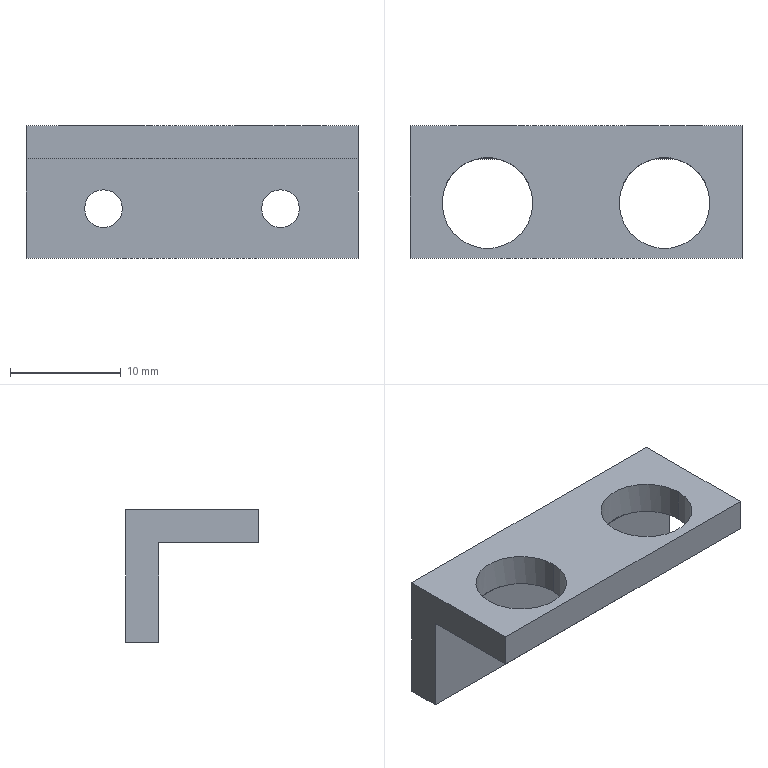Part | NX | 1 solid | 22 faces | box 30 x 12 x 12 mm | volume 1480 mm3 | plane 10 | cylinder 8 | cone 4 | commonest cylinder face diameters 3.4 x4 8.2 x4
STEP:
#1=CARTESIAN_POINT('',(-8.,4.34,-9.2));
#2=VERTEX_POINT('',#1);
#3=CARTESIAN_POINT('',(-8.,4.34,-5.8));
#4=VERTEX_POINT('',#3);
#5=CARTESIAN_POINT('',(-8.,4.34,-7.5));
#6=DIRECTION('',(0.,1.,0.));
#7=DIRECTION('',(0.,0.,1.));
#8=AXIS2_PLACEMENT_3D('',#5,#6,#7);
#9=CIRCLE('',#8,1.7);
#10=EDGE_CURVE('',#2,#4,#9,.T.);
#11=ORIENTED_EDGE('',*,*,#10,.F.);
#12=CARTESIAN_POINT('',(-8.,6.,-10.86));
#13=VERTEX_POINT('',#12);
#14=CARTESIAN_POINT('',(-8.,6.,-10.86));
#15=DIRECTION('',(0.,0.7071,-0.7071));
#16=VECTOR('',#15,1000.);
#17=LINE('',#14,#16);
#18=EDGE_CURVE('',#2,#13,#17,.T.);
#19=ORIENTED_EDGE('',*,*,#18,.T.);
#20=CARTESIAN_POINT('',(-8.,6.,-4.14));
#21=VERTEX_POINT('',#20);
#22=CARTESIAN_POINT('',(-8.,6.,-7.5));
#23=DIRECTION('',(0.,1.,0.));
#24=DIRECTION('',(0.,0.,1.));
#25=AXIS2_PLACEMENT_3D('',#22,#23,#24);
#26=CIRCLE('',#25,3.36);
#27=EDGE_CURVE('',#13,#21,#26,.T.);
#28=ORIENTED_EDGE('',*,*,#27,.T.);
#29=CARTESIAN_POINT('',(-8.,6.,-4.14));
#30=DIRECTION('',(0.,0.7071,0.7071));
#31=VECTOR('',#30,1000.);
#32=LINE('',#29,#31);
#33=EDGE_CURVE('',#4,#21,#32,.T.);
#34=ORIENTED_EDGE('',*,*,#33,.F.);
#35=EDGE_LOOP('',(#11,#19,#28,#34));
#36=FACE_BOUND('',#35,.T.);
#37=CARTESIAN_POINT('',(-8.,6.,-7.5));
#38=DIRECTION('',(0.,1.,0.));
#39=DIRECTION('',(0.,0.,-1.));
#40=AXIS2_PLACEMENT_3D('',#37,#38,#39);
#41=CONICAL_SURFACE('',#40,3.36,0.7854);
#42=ADVANCED_FACE('',(#36),#41,.F.);
#43=CARTESIAN_POINT('',(-8.,3.,-9.2));
#44=VERTEX_POINT('',#43);
#45=CARTESIAN_POINT('',(-8.,3.,-5.8));
#46=VERTEX_POINT('',#45);
#47=CARTESIAN_POINT('',(-8.,3.,-7.5));
#48=DIRECTION('',(0.,1.,0.));
#49=DIRECTION('',(0.,0.,1.));
#50=AXIS2_PLACEMENT_3D('',#47,#48,#49);
#51=CIRCLE('',#50,1.7);
#52=EDGE_CURVE('',#44,#46,#51,.T.);
#53=ORIENTED_EDGE('',*,*,#52,.F.);
#54=CARTESIAN_POINT('',(-8.,6.,-9.2));
#55=DIRECTION('',(0.,1.,0.));
#56=VECTOR('',#55,1000.);
#57=LINE('',#54,#56);
#58=EDGE_CURVE('',#44,#2,#57,.T.);
#59=ORIENTED_EDGE('',*,*,#58,.T.);
#60=ORIENTED_EDGE('',*,*,#10,.T.);
#61=CARTESIAN_POINT('',(-8.,6.,-5.8));
#62=DIRECTION('',(0.,1.,0.));
#63=VECTOR('',#62,1000.);
#64=LINE('',#61,#63);
#65=EDGE_CURVE('',#46,#4,#64,.T.);
#66=ORIENTED_EDGE('',*,*,#65,.F.);
#67=EDGE_LOOP('',(#53,#59,#60,#66));
#68=FACE_BOUND('',#67,.T.);
#69=CARTESIAN_POINT('',(-8.,6.,-7.5));
#70=DIRECTION('',(0.,1.,0.));
#71=DIRECTION('',(0.,0.,-1.));
#72=AXIS2_PLACEMENT_3D('',#69,#70,#71);
#73=CYLINDRICAL_SURFACE('',#72,1.7);
#74=ADVANCED_FACE('',(#68),#73,.F.);
#75=CARTESIAN_POINT('',(8.,4.34,-9.2));
#76=VERTEX_POINT('',#75);
#77=CARTESIAN_POINT('',(8.,4.34,-5.8));
#78=VERTEX_POINT('',#77);
#79=CARTESIAN_POINT('',(8.,4.34,-7.5));
#80=DIRECTION('',(0.,1.,0.));
#81=DIRECTION('',(0.,0.,1.));
#82=AXIS2_PLACEMENT_3D('',#79,#80,#81);
#83=CIRCLE('',#82,1.7);
#84=EDGE_CURVE('',#76,#78,#83,.T.);
#85=ORIENTED_EDGE('',*,*,#84,.F.);
#86=CARTESIAN_POINT('',(8.,6.,-10.86));
#87=VERTEX_POINT('',#86);
#88=CARTESIAN_POINT('',(8.,6.,-10.86));
#89=DIRECTION('',(0.,0.7071,-0.7071));
#90=VECTOR('',#89,1000.);
#91=LINE('',#88,#90);
#92=EDGE_CURVE('',#76,#87,#91,.T.);
#93=ORIENTED_EDGE('',*,*,#92,.T.);
#94=CARTESIAN_POINT('',(8.,6.,-4.14));
#95=VERTEX_POINT('',#94);
#96=CARTESIAN_POINT('',(8.,6.,-7.5));
#97=DIRECTION('',(0.,1.,0.));
#98=DIRECTION('',(0.,0.,1.));
#99=AXIS2_PLACEMENT_3D('',#96,#97,#98);
#100=CIRCLE('',#99,3.36);
#101=EDGE_CURVE('',#87,#95,#100,.T.);
#102=ORIENTED_EDGE('',*,*,#101,.T.);
#103=CARTESIAN_POINT('',(8.,6.,-4.14));
#104=DIRECTION('',(0.,0.7071,0.7071));
#105=VECTOR('',#104,1000.);
#106=LINE('',#103,#105);
#107=EDGE_CURVE('',#78,#95,#106,.T.);
#108=ORIENTED_EDGE('',*,*,#107,.F.);
#109=EDGE_LOOP('',(#85,#93,#102,#108));
#110=FACE_BOUND('',#109,.T.);
#111=CARTESIAN_POINT('',(8.,6.,-7.5));
#112=DIRECTION('',(0.,1.,0.));
#113=DIRECTION('',(0.,0.,-1.));
#114=AXIS2_PLACEMENT_3D('',#111,#112,#113);
#115=CONICAL_SURFACE('',#114,3.36,0.7854);
#116=ADVANCED_FACE('',(#110),#115,.F.);
#117=CARTESIAN_POINT('',(8.,3.,-9.2));
#118=VERTEX_POINT('',#117);
#119=CARTESIAN_POINT('',(8.,3.,-5.8));
#120=VERTEX_POINT('',#119);
#121=CARTESIAN_POINT('',(8.,3.,-7.5));
#122=DIRECTION('',(0.,1.,0.));
#123=DIRECTION('',(0.,0.,1.));
#124=AXIS2_PLACEMENT_3D('',#121,#122,#123);
#125=CIRCLE('',#124,1.7);
#126=EDGE_CURVE('',#118,#120,#125,.T.);
#127=ORIENTED_EDGE('',*,*,#126,.F.);
#128=CARTESIAN_POINT('',(8.,6.,-9.2));
#129=DIRECTION('',(0.,1.,0.));
#130=VECTOR('',#129,1000.);
#131=LINE('',#128,#130);
#132=EDGE_CURVE('',#118,#76,#131,.T.);
#133=ORIENTED_EDGE('',*,*,#132,.T.);
#134=ORIENTED_EDGE('',*,*,#84,.T.);
#135=CARTESIAN_POINT('',(8.,6.,-5.8));
#136=DIRECTION('',(0.,1.,0.));
#137=VECTOR('',#136,1000.);
#138=LINE('',#135,#137);
#139=EDGE_CURVE('',#120,#78,#138,.T.);
#140=ORIENTED_EDGE('',*,*,#139,.F.);
#141=EDGE_LOOP('',(#127,#133,#134,#140));
#142=FACE_BOUND('',#141,.T.);
#143=CARTESIAN_POINT('',(8.,6.,-7.5));
#144=DIRECTION('',(0.,1.,0.));
#145=DIRECTION('',(0.,0.,-1.));
#146=AXIS2_PLACEMENT_3D('',#143,#144,#145);
#147=CYLINDRICAL_SURFACE('',#146,1.7);
#148=ADVANCED_FACE('',(#142),#147,.F.);
#149=CARTESIAN_POINT('',(-12.1,-0.9982,-3.));
#150=VERTEX_POINT('',#149);
#151=CARTESIAN_POINT('',(-3.9,-0.9982,-3.));
#152=VERTEX_POINT('',#151);
#153=CARTESIAN_POINT('',(-8.,-0.9982,-3.));
#154=DIRECTION('',(0.,0.,1.));
#155=DIRECTION('',(1.,0.,0.));
#156=AXIS2_PLACEMENT_3D('',#153,#154,#155);
#157=CIRCLE('',#156,4.1);
#158=EDGE_CURVE('',#150,#152,#157,.T.);
#159=ORIENTED_EDGE('',*,*,#158,.F.);
#160=CARTESIAN_POINT('',(-12.1,-0.9982,0.));
#161=VERTEX_POINT('',#160);
#162=CARTESIAN_POINT('',(-12.1,-0.9982,0.));
#163=DIRECTION('',(0.,0.,1.));
#164=VECTOR('',#163,1000.);
#165=LINE('',#162,#164);
#166=EDGE_CURVE('',#150,#161,#165,.T.);
#167=ORIENTED_EDGE('',*,*,#166,.T.);
#168=CARTESIAN_POINT('',(-3.9,-0.9982,0.));
#169=VERTEX_POINT('',#168);
#170=CARTESIAN_POINT('',(-8.,-0.9982,0.));
#171=DIRECTION('',(0.,0.,1.));
#172=DIRECTION('',(1.,0.,0.));
#173=AXIS2_PLACEMENT_3D('',#170,#171,#172);
#174=CIRCLE('',#173,4.1);
#175=EDGE_CURVE('',#161,#169,#174,.T.);
#176=ORIENTED_EDGE('',*,*,#175,.T.);
#177=CARTESIAN_POINT('',(-3.9,-0.9982,0.));
#178=DIRECTION('',(0.,0.,1.));
#179=VECTOR('',#178,1000.);
#180=LINE('',#177,#179);
#181=EDGE_CURVE('',#152,#169,#180,.T.);
#182=ORIENTED_EDGE('',*,*,#181,.F.);
#183=EDGE_LOOP('',(#159,#167,#176,#182));
#184=FACE_BOUND('',#183,.T.);
#185=CARTESIAN_POINT('',(-8.,-0.9982,0.));
#186=DIRECTION('',(0.,0.,1.));
#187=DIRECTION('',(-1.,0.,0.));
#188=AXIS2_PLACEMENT_3D('',#185,#186,#187);
#189=CYLINDRICAL_SURFACE('',#188,4.1);
#190=ADVANCED_FACE('',(#184),#189,.F.);
#191=CARTESIAN_POINT('',(3.9,-0.9982,-3.));
#192=VERTEX_POINT('',#191);
#193=CARTESIAN_POINT('',(12.1,-0.9982,-3.));
#194=VERTEX_POINT('',#193);
#195=CARTESIAN_POINT('',(8.,-0.9982,-3.));
#196=DIRECTION('',(0.,0.,1.));
#197=DIRECTION('',(1.,0.,0.));
#198=AXIS2_PLACEMENT_3D('',#195,#196,#197);
#199=CIRCLE('',#198,4.1);
#200=EDGE_CURVE('',#192,#194,#199,.T.);
#201=ORIENTED_EDGE('',*,*,#200,.F.);
#202=CARTESIAN_POINT('',(3.9,-0.9982,0.));
#203=VERTEX_POINT('',#202);
#204=CARTESIAN_POINT('',(3.9,-0.9982,0.));
#205=DIRECTION('',(0.,0.,1.));
#206=VECTOR('',#205,1000.);
#207=LINE('',#204,#206);
#208=EDGE_CURVE('',#192,#203,#207,.T.);
#209=ORIENTED_EDGE('',*,*,#208,.T.);
#210=CARTESIAN_POINT('',(12.1,-0.9982,0.));
#211=VERTEX_POINT('',#210);
#212=CARTESIAN_POINT('',(8.,-0.9982,0.));
#213=DIRECTION('',(0.,0.,1.));
#214=DIRECTION('',(1.,0.,0.));
#215=AXIS2_PLACEMENT_3D('',#212,#213,#214);
#216=CIRCLE('',#215,4.1);
#217=EDGE_CURVE('',#203,#211,#216,.T.);
#218=ORIENTED_EDGE('',*,*,#217,.T.);
#219=CARTESIAN_POINT('',(12.1,-0.9982,0.));
#220=DIRECTION('',(0.,0.,1.));
#221=VECTOR('',#220,1000.);
#222=LINE('',#219,#221);
#223=EDGE_CURVE('',#194,#211,#222,.T.);
#224=ORIENTED_EDGE('',*,*,#223,.F.);
#225=EDGE_LOOP('',(#201,#209,#218,#224));
#226=FACE_BOUND('',#225,.T.);
#227=CARTESIAN_POINT('',(8.,-0.9982,0.));
#228=DIRECTION('',(0.,0.,1.));
#229=DIRECTION('',(-1.,0.,0.));
#230=AXIS2_PLACEMENT_3D('',#227,#228,#229);
#231=CYLINDRICAL_SURFACE('',#230,4.1);
#232=ADVANCED_FACE('',(#226),#231,.F.);
#233=CARTESIAN_POINT('',(8.,6.,-7.5));
#234=DIRECTION('',(0.,1.,0.));
#235=DIRECTION('',(0.,0.,1.));
#236=AXIS2_PLACEMENT_3D('',#233,#234,#235);
#237=CIRCLE('',#236,3.36);
#238=EDGE_CURVE('',#95,#87,#237,.T.);
#239=ORIENTED_EDGE('',*,*,#238,.F.);
#240=ORIENTED_EDGE('',*,*,#101,.F.);
#241=EDGE_LOOP('',(#239,#240));
#242=FACE_BOUND('',#241,.T.);
#243=CARTESIAN_POINT('',(-15.,6.,-12.));
#244=VERTEX_POINT('',#243);
#245=CARTESIAN_POINT('',(-15.,6.,0.));
#246=VERTEX_POINT('',#245);
#247=CARTESIAN_POINT('',(-15.,6.,-12.));
#248=DIRECTION('',(0.,0.,1.));
#249=VECTOR('',#248,1000.);
#250=LINE('',#247,#249);
#251=EDGE_CURVE('',#244,#246,#250,.T.);
#252=ORIENTED_EDGE('',*,*,#251,.T.);
#253=CARTESIAN_POINT('',(15.,6.,0.));
#254=VERTEX_POINT('',#253);
#255=CARTESIAN_POINT('',(15.,6.,0.));
#256=DIRECTION('',(-1.,0.,0.));
#257=VECTOR('',#256,1000.);
#258=LINE('',#255,#257);
#259=EDGE_CURVE('',#254,#246,#258,.T.);
#260=ORIENTED_EDGE('',*,*,#259,.F.);
#261=CARTESIAN_POINT('',(15.,6.,-12.));
#262=VERTEX_POINT('',#261);
#263=CARTESIAN_POINT('',(15.,6.,-12.));
#264=DIRECTION('',(0.,0.,1.));
#265=VECTOR('',#264,1000.);
#266=LINE('',#263,#265);
#267=EDGE_CURVE('',#262,#254,#266,.T.);
#268=ORIENTED_EDGE('',*,*,#267,.F.);
#269=CARTESIAN_POINT('',(15.,6.,-12.));
#270=DIRECTION('',(-1.,0.,0.));
#271=VECTOR('',#270,1000.);
#272=LINE('',#269,#271);
#273=EDGE_CURVE('',#262,#244,#272,.T.);
#274=ORIENTED_EDGE('',*,*,#273,.T.);
#275=EDGE_LOOP('',(#252,#260,#268,#274));
#276=FACE_BOUND('',#275,.T.);
#277=CARTESIAN_POINT('',(-8.,6.,-7.5));
#278=DIRECTION('',(0.,1.,0.));
#279=DIRECTION('',(0.,0.,1.));
#280=AXIS2_PLACEMENT_3D('',#277,#278,#279);
#281=CIRCLE('',#280,3.36);
#282=EDGE_CURVE('',#21,#13,#281,.T.);
#283=ORIENTED_EDGE('',*,*,#282,.F.);
#284=ORIENTED_EDGE('',*,*,#27,.F.);
#285=EDGE_LOOP('',(#283,#284));
#286=FACE_BOUND('',#285,.T.);
#287=CARTESIAN_POINT('',(15.,6.,-12.));
#288=DIRECTION('',(0.,-1.,0.));
#289=DIRECTION('',(0.,0.,1.));
#290=AXIS2_PLACEMENT_3D('',#287,#288,#289);
#291=PLANE('',#290);
#292=ADVANCED_FACE('',(#242,#276,#286),#291,.F.);
#293=CARTESIAN_POINT('',(-8.908,3.,-3.));
#294=VERTEX_POINT('',#293);
#295=CARTESIAN_POINT('',(-15.,3.,-3.));
#296=VERTEX_POINT('',#295);
#297=CARTESIAN_POINT('',(15.,3.,-3.));
#298=DIRECTION('',(-1.,0.,0.));
#299=VECTOR('',#298,1000.);
#300=LINE('',#297,#299);
#301=EDGE_CURVE('',#294,#296,#300,.T.);
#302=ORIENTED_EDGE('',*,*,#301,.F.);
#303=CARTESIAN_POINT('',(-8.,-0.9982,-3.));
#304=DIRECTION('',(0.,0.,1.));
#305=DIRECTION('',(1.,0.,0.));
#306=AXIS2_PLACEMENT_3D('',#303,#304,#305);
#307=CIRCLE('',#306,4.1);
#308=EDGE_CURVE('',#294,#150,#307,.T.);
#309=ORIENTED_EDGE('',*,*,#308,.T.);
#310=ORIENTED_EDGE('',*,*,#158,.T.);
#311=CARTESIAN_POINT('',(-7.092,3.,-3.));
#312=VERTEX_POINT('',#311);
#313=CARTESIAN_POINT('',(-8.,-0.9982,-3.));
#314=DIRECTION('',(0.,0.,1.));
#315=DIRECTION('',(1.,0.,0.));
#316=AXIS2_PLACEMENT_3D('',#313,#314,#315);
#317=CIRCLE('',#316,4.1);
#318=EDGE_CURVE('',#152,#312,#317,.T.);
#319=ORIENTED_EDGE('',*,*,#318,.T.);
#320=CARTESIAN_POINT('',(7.092,3.,-3.));
#321=VERTEX_POINT('',#320);
#322=CARTESIAN_POINT('',(15.,3.,-3.));
#323=DIRECTION('',(-1.,0.,0.));
#324=VECTOR('',#323,1000.);
#325=LINE('',#322,#324);
#326=EDGE_CURVE('',#321,#312,#325,.T.);
#327=ORIENTED_EDGE('',*,*,#326,.F.);
#328=CARTESIAN_POINT('',(8.,-0.9982,-3.));
#329=DIRECTION('',(0.,0.,1.));
#330=DIRECTION('',(1.,0.,0.));
#331=AXIS2_PLACEMENT_3D('',#328,#329,#330);
#332=CIRCLE('',#331,4.1);
#333=EDGE_CURVE('',#321,#192,#332,.T.);
#334=ORIENTED_EDGE('',*,*,#333,.T.);
#335=ORIENTED_EDGE('',*,*,#200,.T.);
#336=CARTESIAN_POINT('',(8.908,3.,-3.));
#337=VERTEX_POINT('',#336);
#338=CARTESIAN_POINT('',(8.,-0.9982,-3.));
#339=DIRECTION('',(0.,0.,1.));
#340=DIRECTION('',(1.,0.,0.));
#341=AXIS2_PLACEMENT_3D('',#338,#339,#340);
#342=CIRCLE('',#341,4.1);
#343=EDGE_CURVE('',#194,#337,#342,.T.);
#344=ORIENTED_EDGE('',*,*,#343,.T.);
#345=CARTESIAN_POINT('',(15.,3.,-3.));
#346=VERTEX_POINT('',#345);
#347=CARTESIAN_POINT('',(15.,3.,-3.));
#348=DIRECTION('',(-1.,0.,0.));
#349=VECTOR('',#348,1000.);
#350=LINE('',#347,#349);
#351=EDGE_CURVE('',#346,#337,#350,.T.);
#352=ORIENTED_EDGE('',*,*,#351,.F.);
#353=CARTESIAN_POINT('',(15.,-6.,-3.));
#354=VERTEX_POINT('',#353);
#355=CARTESIAN_POINT('',(15.,-6.,-3.));
#356=DIRECTION('',(0.,1.,0.));
#357=VECTOR('',#356,1000.);
#358=LINE('',#355,#357);
#359=EDGE_CURVE('',#354,#346,#358,.T.);
#360=ORIENTED_EDGE('',*,*,#359,.F.);
#361=CARTESIAN_POINT('',(-15.,-6.,-3.));
#362=VERTEX_POINT('',#361);
#363=CARTESIAN_POINT('',(15.,-6.,-3.));
#364=DIRECTION('',(-1.,0.,0.));
#365=VECTOR('',#364,1000.);
#366=LINE('',#363,#365);
#367=EDGE_CURVE('',#354,#362,#366,.T.);
#368=ORIENTED_EDGE('',*,*,#367,.T.);
#369=CARTESIAN_POINT('',(-15.,-6.,-3.));
#370=DIRECTION('',(0.,1.,0.));
#371=VECTOR('',#370,1000.);
#372=LINE('',#369,#371);
#373=EDGE_CURVE('',#362,#296,#372,.T.);
#374=ORIENTED_EDGE('',*,*,#373,.T.);
#375=EDGE_LOOP('',(#302,#309,#310,#319,#327,#334,#335,#344,#352,#360,#368,#374));
#376=FACE_BOUND('',#375,.T.);
#377=CARTESIAN_POINT('',(15.,-6.,-3.));
#378=DIRECTION('',(0.,0.,1.));
#379=DIRECTION('',(-1.,0.,0.));
#380=AXIS2_PLACEMENT_3D('',#377,#378,#379);
#381=PLANE('',#380);
#382=ADVANCED_FACE('',(#376),#381,.F.);
#383=CARTESIAN_POINT('',(-8.,3.,-7.5));
#384=DIRECTION('',(0.,1.,0.));
#385=DIRECTION('',(0.,0.,1.));
#386=AXIS2_PLACEMENT_3D('',#383,#384,#385);
#387=CIRCLE('',#386,1.7);
#388=EDGE_CURVE('',#46,#44,#387,.T.);
#389=ORIENTED_EDGE('',*,*,#388,.T.);
#390=ORIENTED_EDGE('',*,*,#52,.T.);
#391=EDGE_LOOP('',(#389,#390));
#392=FACE_BOUND('',#391,.T.);
#393=CARTESIAN_POINT('',(8.,3.,-7.5));
#394=DIRECTION('',(0.,1.,0.));
#395=DIRECTION('',(0.,0.,1.));
#396=AXIS2_PLACEMENT_3D('',#393,#394,#395);
#397=CIRCLE('',#396,1.7);
#398=EDGE_CURVE('',#120,#118,#397,.T.);
#399=ORIENTED_EDGE('',*,*,#398,.T.);
#400=ORIENTED_EDGE('',*,*,#126,.T.);
#401=EDGE_LOOP('',(#399,#400));
#402=FACE_BOUND('',#401,.T.);
#403=CARTESIAN_POINT('',(-15.,3.,-12.));
#404=VERTEX_POINT('',#403);
#405=CARTESIAN_POINT('',(-15.,3.,-3.));
#406=DIRECTION('',(0.,0.,-1.));
#407=VECTOR('',#406,1000.);
#408=LINE('',#405,#407);
#409=EDGE_CURVE('',#296,#404,#408,.T.);
#410=ORIENTED_EDGE('',*,*,#409,.T.);
#411=CARTESIAN_POINT('',(15.,3.,-12.));
#412=VERTEX_POINT('',#411);
#413=CARTESIAN_POINT('',(15.,3.,-12.));
#414=DIRECTION('',(-1.,0.,0.));
#415=VECTOR('',#414,1000.);
#416=LINE('',#413,#415);
#417=EDGE_CURVE('',#412,#404,#416,.T.);
#418=ORIENTED_EDGE('',*,*,#417,.F.);
#419=CARTESIAN_POINT('',(15.,3.,-3.));
#420=DIRECTION('',(0.,0.,-1.));
#421=VECTOR('',#420,1000.);
#422=LINE('',#419,#421);
#423=EDGE_CURVE('',#346,#412,#422,.T.);
#424=ORIENTED_EDGE('',*,*,#423,.F.);
#425=ORIENTED_EDGE('',*,*,#351,.T.);
#426=CARTESIAN_POINT('',(15.,3.,-3.));
#427=DIRECTION('',(-1.,0.,0.));
#428=VECTOR('',#427,1000.);
#429=LINE('',#426,#428);
#430=EDGE_CURVE('',#337,#321,#429,.T.);
#431=ORIENTED_EDGE('',*,*,#430,.T.);
#432=ORIENTED_EDGE('',*,*,#326,.T.);
#433=CARTESIAN_POINT('',(15.,3.,-3.));
#434=DIRECTION('',(-1.,0.,0.));
#435=VECTOR('',#434,1000.);
#436=LINE('',#433,#435);
#437=EDGE_CURVE('',#312,#294,#436,.T.);
#438=ORIENTED_EDGE('',*,*,#437,.T.);
#439=ORIENTED_EDGE('',*,*,#301,.T.);
#440=EDGE_LOOP('',(#410,#418,#424,#425,#431,#432,#438,#439));
#441=FACE_BOUND('',#440,.T.);
#442=CARTESIAN_POINT('',(15.,3.,-3.));
#443=DIRECTION('',(0.,1.,0.));
#444=DIRECTION('',(0.,0.,-1.));
#445=AXIS2_PLACEMENT_3D('',#442,#443,#444);
#446=PLANE('',#445);
#447=ADVANCED_FACE('',(#392,#402,#441),#446,.F.);
#448=CARTESIAN_POINT('',(-15.,3.,-12.));
#449=DIRECTION('',(0.,1.,0.));
#450=VECTOR('',#449,1000.);
#451=LINE('',#448,#450);
#452=EDGE_CURVE('',#404,#244,#451,.T.);
#453=ORIENTED_EDGE('',*,*,#452,.T.);
#454=ORIENTED_EDGE('',*,*,#273,.F.);
#455=CARTESIAN_POINT('',(15.,3.,-12.));
#456=DIRECTION('',(0.,1.,0.));
#457=VECTOR('',#456,1000.);
#458=LINE('',#455,#457);
#459=EDGE_CURVE('',#412,#262,#458,.T.);
#460=ORIENTED_EDGE('',*,*,#459,.F.);
#461=ORIENTED_EDGE('',*,*,#417,.T.);
#462=EDGE_LOOP('',(#453,#454,#460,#461));
#463=FACE_BOUND('',#462,.T.);
#464=CARTESIAN_POINT('',(15.,3.,-12.));
#465=DIRECTION('',(0.,0.,1.));
#466=DIRECTION('',(0.,1.,0.));
#467=AXIS2_PLACEMENT_3D('',#464,#465,#466);
#468=PLANE('',#467);
#469=ADVANCED_FACE('',(#463),#468,.F.);
#470=CARTESIAN_POINT('',(-8.,-0.9982,0.));
#471=DIRECTION('',(0.,0.,1.));
#472=DIRECTION('',(1.,0.,0.));
#473=AXIS2_PLACEMENT_3D('',#470,#471,#472);
#474=CIRCLE('',#473,4.1);
#475=EDGE_CURVE('',#169,#161,#474,.T.);
#476=ORIENTED_EDGE('',*,*,#475,.F.);
#477=ORIENTED_EDGE('',*,*,#175,.F.);
#478=EDGE_LOOP('',(#476,#477));
#479=FACE_BOUND('',#478,.T.);
#480=CARTESIAN_POINT('',(8.,-0.9982,0.));
#481=DIRECTION('',(0.,0.,1.));
#482=DIRECTION('',(1.,0.,0.));
#483=AXIS2_PLACEMENT_3D('',#480,#481,#482);
#484=CIRCLE('',#483,4.1);
#485=EDGE_CURVE('',#211,#203,#484,.T.);
#486=ORIENTED_EDGE('',*,*,#485,.F.);
#487=ORIENTED_EDGE('',*,*,#217,.F.);
#488=EDGE_LOOP('',(#486,#487));
#489=FACE_BOUND('',#488,.T.);
#490=CARTESIAN_POINT('',(-15.,-6.,0.));
#491=VERTEX_POINT('',#490);
#492=CARTESIAN_POINT('',(-15.,6.,0.));
#493=DIRECTION('',(0.,-1.,0.));
#494=VECTOR('',#493,1000.);
#495=LINE('',#492,#494);
#496=EDGE_CURVE('',#246,#491,#495,.T.);
#497=ORIENTED_EDGE('',*,*,#496,.T.);
#498=CARTESIAN_POINT('',(15.,-6.,0.));
#499=VERTEX_POINT('',#498);
#500=CARTESIAN_POINT('',(15.,-6.,0.));
#501=DIRECTION('',(-1.,0.,0.));
#502=VECTOR('',#501,1000.);
#503=LINE('',#500,#502);
#504=EDGE_CURVE('',#499,#491,#503,.T.);
#505=ORIENTED_EDGE('',*,*,#504,.F.);
#506=CARTESIAN_POINT('',(15.,6.,0.));
#507=DIRECTION('',(0.,-1.,0.));
#508=VECTOR('',#507,1000.);
#509=LINE('',#506,#508);
#510=EDGE_CURVE('',#254,#499,#509,.T.);
#511=ORIENTED_EDGE('',*,*,#510,.F.);
#512=ORIENTED_EDGE('',*,*,#259,.T.);
#513=EDGE_LOOP('',(#497,#505,#511,#512));
#514=FACE_BOUND('',#513,.T.);
#515=CARTESIAN_POINT('',(15.,6.,0.));
#516=DIRECTION('',(0.,0.,-1.));
#517=DIRECTION('',(0.,-1.,0.));
#518=AXIS2_PLACEMENT_3D('',#515,#516,#517);
#519=PLANE('',#518);
#520=ADVANCED_FACE('',(#479,#489,#514),#519,.F.);
#521=CARTESIAN_POINT('',(-15.,-6.,0.));
#522=DIRECTION('',(0.,0.,-1.));
#523=VECTOR('',#522,1000.);
#524=LINE('',#521,#523);
#525=EDGE_CURVE('',#491,#362,#524,.T.);
#526=ORIENTED_EDGE('',*,*,#525,.T.);
#527=ORIENTED_EDGE('',*,*,#367,.F.);
#528=CARTESIAN_POINT('',(15.,-6.,0.));
#529=DIRECTION('',(0.,0.,-1.));
#530=VECTOR('',#529,1000.);
#531=LINE('',#528,#530);
#532=EDGE_CURVE('',#499,#354,#531,.T.);
#533=ORIENTED_EDGE('',*,*,#532,.F.);
#534=ORIENTED_EDGE('',*,*,#504,.T.);
#535=EDGE_LOOP('',(#526,#527,#533,#534));
#536=FACE_BOUND('',#535,.T.);
#537=CARTESIAN_POINT('',(15.,-6.,0.));
#538=DIRECTION('',(0.,1.,0.));
#539=DIRECTION('',(0.,0.,-1.));
#540=AXIS2_PLACEMENT_3D('',#537,#538,#539);
#541=PLANE('',#540);
#542=ADVANCED_FACE('',(#536),#541,.F.);
#543=ORIENTED_EDGE('',*,*,#359,.T.);
#544=ORIENTED_EDGE('',*,*,#423,.T.);
#545=ORIENTED_EDGE('',*,*,#459,.T.);
#546=ORIENTED_EDGE('',*,*,#267,.T.);
#547=ORIENTED_EDGE('',*,*,#510,.T.);
#548=ORIENTED_EDGE('',*,*,#532,.T.);
#549=EDGE_LOOP('',(#543,#544,#545,#546,#547,#548));
#550=FACE_BOUND('',#549,.T.);
#551=CARTESIAN_POINT('',(15.,3.,-3.));
#552=DIRECTION('',(-1.,0.,0.));
#553=DIRECTION('',(0.,0.,-1.));
#554=AXIS2_PLACEMENT_3D('',#551,#552,#553);
#555=PLANE('',#554);
#556=ADVANCED_FACE('',(#550),#555,.F.);
#557=ORIENTED_EDGE('',*,*,#373,.F.);
#558=ORIENTED_EDGE('',*,*,#525,.F.);
#559=ORIENTED_EDGE('',*,*,#496,.F.);
#560=ORIENTED_EDGE('',*,*,#251,.F.);
#561=ORIENTED_EDGE('',*,*,#452,.F.);
#562=ORIENTED_EDGE('',*,*,#409,.F.);
#563=EDGE_LOOP('',(#557,#558,#559,#560,#561,#562));
#564=FACE_BOUND('',#563,.T.);
#565=CARTESIAN_POINT('',(-15.,3.,-3.));
#566=DIRECTION('',(-1.,0.,0.));
#567=DIRECTION('',(0.,0.,-1.));
#568=AXIS2_PLACEMENT_3D('',#565,#566,#567);
#569=PLANE('',#568);
#570=ADVANCED_FACE('',(#564),#569,.T.);
#571=ORIENTED_EDGE('',*,*,#208,.F.);
#572=ORIENTED_EDGE('',*,*,#333,.F.);
#573=CARTESIAN_POINT('',(8.,-0.9982,-3.));
#574=DIRECTION('',(0.,0.,-1.));
#575=DIRECTION('',(1.,0.,0.));
#576=AXIS2_PLACEMENT_3D('',#573,#574,#575);
#577=CIRCLE('',#576,4.1);
#578=EDGE_CURVE('',#321,#337,#577,.T.);
#579=ORIENTED_EDGE('',*,*,#578,.T.);
#580=ORIENTED_EDGE('',*,*,#343,.F.);
#581=ORIENTED_EDGE('',*,*,#223,.T.);
#582=ORIENTED_EDGE('',*,*,#485,.T.);
#583=EDGE_LOOP('',(#571,#572,#579,#580,#581,#582));
#584=FACE_BOUND('',#583,.T.);
#585=CARTESIAN_POINT('',(8.,-0.9982,0.));
#586=DIRECTION('',(0.,0.,1.));
#587=DIRECTION('',(-1.,0.,0.));
#588=AXIS2_PLACEMENT_3D('',#585,#586,#587);
#589=CYLINDRICAL_SURFACE('',#588,4.1);
#590=ADVANCED_FACE('',(#584),#589,.F.);
#591=ORIENTED_EDGE('',*,*,#578,.F.);
#592=ORIENTED_EDGE('',*,*,#430,.F.);
#593=EDGE_LOOP('',(#591,#592));
#594=FACE_BOUND('',#593,.T.);
#595=CARTESIAN_POINT('',(15.,-6.,-3.));
#596=DIRECTION('',(0.,0.,1.));
#597=DIRECTION('',(-1.,0.,0.));
#598=AXIS2_PLACEMENT_3D('',#595,#596,#597);
#599=PLANE('',#598);
#600=ADVANCED_FACE('',(#594),#599,.T.);
#601=ORIENTED_EDGE('',*,*,#166,.F.);
#602=ORIENTED_EDGE('',*,*,#308,.F.);
#603=CARTESIAN_POINT('',(-8.,-0.9982,-3.));
#604=DIRECTION('',(0.,0.,-1.));
#605=DIRECTION('',(1.,0.,0.));
#606=AXIS2_PLACEMENT_3D('',#603,#604,#605);
#607=CIRCLE('',#606,4.1);
#608=EDGE_CURVE('',#294,#312,#607,.T.);
#609=ORIENTED_EDGE('',*,*,#608,.T.);
#610=ORIENTED_EDGE('',*,*,#318,.F.);
#611=ORIENTED_EDGE('',*,*,#181,.T.);
#612=ORIENTED_EDGE('',*,*,#475,.T.);
#613=EDGE_LOOP('',(#601,#602,#609,#610,#611,#612));
#614=FACE_BOUND('',#613,.T.);
#615=CARTESIAN_POINT('',(-8.,-0.9982,0.));
#616=DIRECTION('',(0.,0.,1.));
#617=DIRECTION('',(-1.,0.,0.));
#618=AXIS2_PLACEMENT_3D('',#615,#616,#617);
#619=CYLINDRICAL_SURFACE('',#618,4.1);
#620=ADVANCED_FACE('',(#614),#619,.F.);
#621=ORIENTED_EDGE('',*,*,#608,.F.);
#622=ORIENTED_EDGE('',*,*,#437,.F.);
#623=EDGE_LOOP('',(#621,#622));
#624=FACE_BOUND('',#623,.T.);
#625=CARTESIAN_POINT('',(15.,-6.,-3.));
#626=DIRECTION('',(0.,0.,1.));
#627=DIRECTION('',(-1.,0.,0.));
#628=AXIS2_PLACEMENT_3D('',#625,#626,#627);
#629=PLANE('',#628);
#630=ADVANCED_FACE('',(#624),#629,.T.);
#631=ORIENTED_EDGE('',*,*,#132,.F.);
#632=ORIENTED_EDGE('',*,*,#398,.F.);
#633=ORIENTED_EDGE('',*,*,#139,.T.);
#634=CARTESIAN_POINT('',(8.,4.34,-7.5));
#635=DIRECTION('',(0.,1.,0.));
#636=DIRECTION('',(0.,0.,1.));
#637=AXIS2_PLACEMENT_3D('',#634,#635,#636);
#638=CIRCLE('',#637,1.7);
#639=EDGE_CURVE('',#78,#76,#638,.T.);
#640=ORIENTED_EDGE('',*,*,#639,.T.);
#641=EDGE_LOOP('',(#631,#632,#633,#640));
#642=FACE_BOUND('',#641,.T.);
#643=CARTESIAN_POINT('',(8.,6.,-7.5));
#644=DIRECTION('',(0.,1.,0.));
#645=DIRECTION('',(0.,0.,-1.));
#646=AXIS2_PLACEMENT_3D('',#643,#644,#645);
#647=CYLINDRICAL_SURFACE('',#646,1.7);
#648=ADVANCED_FACE('',(#642),#647,.F.);
#649=ORIENTED_EDGE('',*,*,#92,.F.);
#650=ORIENTED_EDGE('',*,*,#639,.F.);
#651=ORIENTED_EDGE('',*,*,#107,.T.);
#652=ORIENTED_EDGE('',*,*,#238,.T.);
#653=EDGE_LOOP('',(#649,#650,#651,#652));
#654=FACE_BOUND('',#653,.T.);
#655=CARTESIAN_POINT('',(8.,6.,-7.5));
#656=DIRECTION('',(0.,1.,0.));
#657=DIRECTION('',(0.,0.,-1.));
#658=AXIS2_PLACEMENT_3D('',#655,#656,#657);
#659=CONICAL_SURFACE('',#658,3.36,0.7854);
#660=ADVANCED_FACE('',(#654),#659,.F.);
#661=ORIENTED_EDGE('',*,*,#58,.F.);
#662=ORIENTED_EDGE('',*,*,#388,.F.);
#663=ORIENTED_EDGE('',*,*,#65,.T.);
#664=CARTESIAN_POINT('',(-8.,4.34,-7.5));
#665=DIRECTION('',(0.,1.,0.));
#666=DIRECTION('',(0.,0.,1.));
#667=AXIS2_PLACEMENT_3D('',#664,#665,#666);
#668=CIRCLE('',#667,1.7);
#669=EDGE_CURVE('',#4,#2,#668,.T.);
#670=ORIENTED_EDGE('',*,*,#669,.T.);
#671=EDGE_LOOP('',(#661,#662,#663,#670));
#672=FACE_BOUND('',#671,.T.);
#673=CARTESIAN_POINT('',(-8.,6.,-7.5));
#674=DIRECTION('',(0.,1.,0.));
#675=DIRECTION('',(0.,0.,-1.));
#676=AXIS2_PLACEMENT_3D('',#673,#674,#675);
#677=CYLINDRICAL_SURFACE('',#676,1.7);
#678=ADVANCED_FACE('',(#672),#677,.F.);
#679=ORIENTED_EDGE('',*,*,#18,.F.);
#680=ORIENTED_EDGE('',*,*,#669,.F.);
#681=ORIENTED_EDGE('',*,*,#33,.T.);
#682=ORIENTED_EDGE('',*,*,#282,.T.);
#683=EDGE_LOOP('',(#679,#680,#681,#682));
#684=FACE_BOUND('',#683,.T.);
#685=CARTESIAN_POINT('',(-8.,6.,-7.5));
#686=DIRECTION('',(0.,1.,0.));
#687=DIRECTION('',(0.,0.,-1.));
#688=AXIS2_PLACEMENT_3D('',#685,#686,#687);
#689=CONICAL_SURFACE('',#688,3.36,0.7854);
#690=ADVANCED_FACE('',(#684),#689,.F.);
#691=CLOSED_SHELL('',(#42,#74,#116,#148,#190,#232,#292,#382,#447,#469,#520,#542,#556,#570,#590,#600,#620,#630,#648,#660,#678,#690));
#692=MANIFOLD_SOLID_BREP('',#691);
#693=(LENGTH_UNIT()NAMED_UNIT(*)SI_UNIT(.MILLI.,.METRE.));
#694=UNCERTAINTY_MEASURE_WITH_UNIT(LENGTH_MEASURE(0.00001),#693,'','');
#695=(NAMED_UNIT(*)PLANE_ANGLE_UNIT()SI_UNIT($,.RADIAN.));
#696=(NAMED_UNIT(*)SI_UNIT($,.STERADIAN.)SOLID_ANGLE_UNIT());
#697=(GEOMETRIC_REPRESENTATION_CONTEXT(3)GLOBAL_UNCERTAINTY_ASSIGNED_CONTEXT((#694))GLOBAL_UNIT_ASSIGNED_CONTEXT((#693,#695,#696))REPRESENTATION_CONTEXT('',''));
#698=ADVANCED_BREP_SHAPE_REPRESENTATION('',(#692),#697);